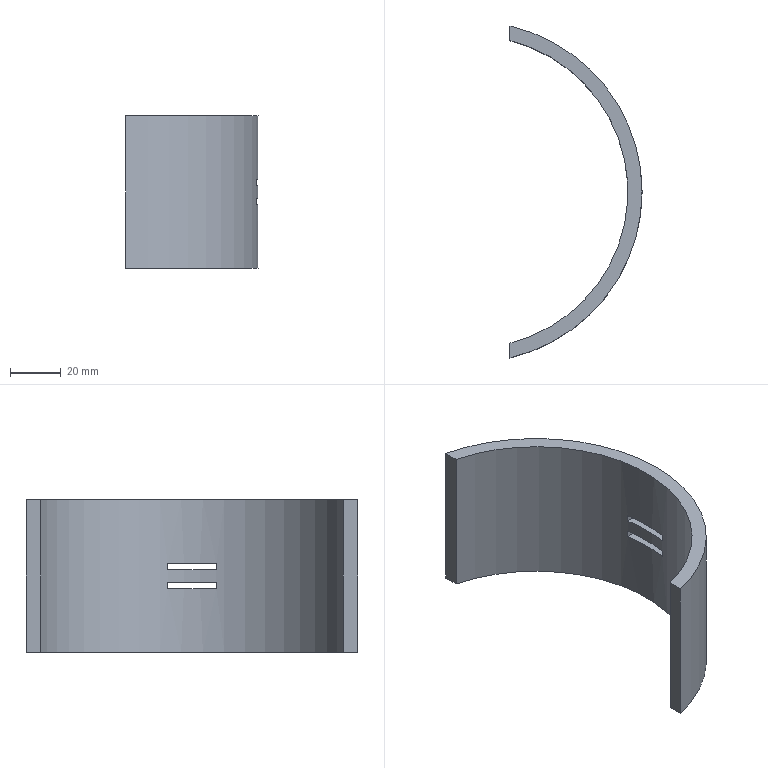Part | SolidWorks | features Extrusion 1, ICE 1 | 1 solid | 14 faces | box 51.978 x 130.553 x 60 mm | volume 56854 mm3 | plane 12 | cylinder 2 | commonest cylinder face diameters 122.792 x1 133.955 x1
STEP:
#1=CARTESIAN_POINT('',(66.293,-9.55,27.496));
#2=VERTEX_POINT('',#1);
#3=CARTESIAN_POINT('',(66.293,-9.55,24.996));
#4=VERTEX_POINT('',#3);
#5=CARTESIAN_POINT('',(66.293,-9.55,60.));
#6=DIRECTION('',(0.,0.,-1.));
#7=VECTOR('',#6,1000.);
#8=LINE('',#5,#7);
#9=EDGE_CURVE('',#2,#4,#8,.T.);
#10=ORIENTED_EDGE('',*,*,#9,.F.);
#11=CARTESIAN_POINT('',(66.293,9.55,27.496));
#12=VERTEX_POINT('',#11);
#13=CARTESIAN_POINT('',(0.,0.,27.496));
#14=DIRECTION('',(0.,0.,-1.));
#15=DIRECTION('',(-1.,0.,0.));
#16=AXIS2_PLACEMENT_3D('',#13,#14,#15);
#17=CIRCLE('',#16,66.978);
#18=EDGE_CURVE('',#12,#2,#17,.T.);
#19=ORIENTED_EDGE('',*,*,#18,.F.);
#20=CARTESIAN_POINT('',(66.293,9.55,24.996));
#21=VERTEX_POINT('',#20);
#22=CARTESIAN_POINT('',(66.293,9.55,60.));
#23=DIRECTION('',(0.,0.,1.));
#24=VECTOR('',#23,1000.);
#25=LINE('',#22,#24);
#26=EDGE_CURVE('',#21,#12,#25,.T.);
#27=ORIENTED_EDGE('',*,*,#26,.F.);
#28=CARTESIAN_POINT('',(0.,0.,24.996));
#29=DIRECTION('',(0.,0.,1.));
#30=DIRECTION('',(1.,0.,0.));
#31=AXIS2_PLACEMENT_3D('',#28,#29,#30);
#32=CIRCLE('',#31,66.978);
#33=EDGE_CURVE('',#4,#21,#32,.T.);
#34=ORIENTED_EDGE('',*,*,#33,.F.);
#35=EDGE_LOOP('',(#10,#19,#27,#34));
#36=FACE_BOUND('',#35,.T.);
#37=CARTESIAN_POINT('',(15.,-65.276,0.));
#38=VERTEX_POINT('',#37);
#39=CARTESIAN_POINT('',(15.,65.276,0.));
#40=VERTEX_POINT('',#39);
#41=CARTESIAN_POINT('',(0.,0.,0.));
#42=DIRECTION('',(0.,0.,1.));
#43=DIRECTION('',(1.,0.,0.));
#44=AXIS2_PLACEMENT_3D('',#41,#42,#43);
#45=CIRCLE('',#44,66.978);
#46=EDGE_CURVE('',#38,#40,#45,.T.);
#47=ORIENTED_EDGE('',*,*,#46,.T.);
#48=CARTESIAN_POINT('',(15.,65.276,60.));
#49=VERTEX_POINT('',#48);
#50=CARTESIAN_POINT('',(15.,65.276,60.));
#51=DIRECTION('',(0.,0.,-1.));
#52=VECTOR('',#51,1000.);
#53=LINE('',#50,#52);
#54=EDGE_CURVE('',#49,#40,#53,.T.);
#55=ORIENTED_EDGE('',*,*,#54,.F.);
#56=CARTESIAN_POINT('',(15.,-65.276,60.));
#57=VERTEX_POINT('',#56);
#58=CARTESIAN_POINT('',(0.,0.,60.));
#59=DIRECTION('',(0.,0.,1.));
#60=DIRECTION('',(1.,0.,0.));
#61=AXIS2_PLACEMENT_3D('',#58,#59,#60);
#62=CIRCLE('',#61,66.978);
#63=EDGE_CURVE('',#57,#49,#62,.T.);
#64=ORIENTED_EDGE('',*,*,#63,.F.);
#65=CARTESIAN_POINT('',(15.,-65.276,60.));
#66=DIRECTION('',(0.,0.,-1.));
#67=VECTOR('',#66,1000.);
#68=LINE('',#65,#67);
#69=EDGE_CURVE('',#57,#38,#68,.T.);
#70=ORIENTED_EDGE('',*,*,#69,.T.);
#71=EDGE_LOOP('',(#47,#55,#64,#70));
#72=FACE_OUTER_BOUND('',#71,.T.);
#73=CARTESIAN_POINT('',(66.293,-9.55,35.004));
#74=VERTEX_POINT('',#73);
#75=CARTESIAN_POINT('',(66.293,-9.55,32.504));
#76=VERTEX_POINT('',#75);
#77=CARTESIAN_POINT('',(66.293,-9.55,60.));
#78=DIRECTION('',(0.,0.,-1.));
#79=VECTOR('',#78,1000.);
#80=LINE('',#77,#79);
#81=EDGE_CURVE('',#74,#76,#80,.T.);
#82=ORIENTED_EDGE('',*,*,#81,.F.);
#83=CARTESIAN_POINT('',(66.293,9.55,35.004));
#84=VERTEX_POINT('',#83);
#85=CARTESIAN_POINT('',(0.,0.,35.004));
#86=DIRECTION('',(0.,0.,-1.));
#87=DIRECTION('',(-1.,0.,0.));
#88=AXIS2_PLACEMENT_3D('',#85,#86,#87);
#89=CIRCLE('',#88,66.978);
#90=EDGE_CURVE('',#84,#74,#89,.T.);
#91=ORIENTED_EDGE('',*,*,#90,.F.);
#92=CARTESIAN_POINT('',(66.293,9.55,32.504));
#93=VERTEX_POINT('',#92);
#94=CARTESIAN_POINT('',(66.293,9.55,60.));
#95=DIRECTION('',(0.,0.,1.));
#96=VECTOR('',#95,1000.);
#97=LINE('',#94,#96);
#98=EDGE_CURVE('',#93,#84,#97,.T.);
#99=ORIENTED_EDGE('',*,*,#98,.F.);
#100=CARTESIAN_POINT('',(0.,0.,32.504));
#101=DIRECTION('',(0.,0.,1.));
#102=DIRECTION('',(1.,0.,0.));
#103=AXIS2_PLACEMENT_3D('',#100,#101,#102);
#104=CIRCLE('',#103,66.978);
#105=EDGE_CURVE('',#76,#93,#104,.T.);
#106=ORIENTED_EDGE('',*,*,#105,.F.);
#107=EDGE_LOOP('',(#82,#91,#99,#106));
#108=FACE_BOUND('',#107,.T.);
#109=CARTESIAN_POINT('',(0.,0.,60.));
#110=DIRECTION('',(0.,0.,-1.));
#111=DIRECTION('',(-1.,0.,0.));
#112=AXIS2_PLACEMENT_3D('',#109,#110,#111);
#113=CYLINDRICAL_SURFACE('',#112,66.978);
#114=ADVANCED_FACE('',(#36,#72,#108),#113,.T.);
#115=CARTESIAN_POINT('',(60.649,-9.55,24.996));
#116=VERTEX_POINT('',#115);
#117=CARTESIAN_POINT('',(60.649,-9.55,27.496));
#118=VERTEX_POINT('',#117);
#119=CARTESIAN_POINT('',(60.649,-9.55,60.));
#120=DIRECTION('',(0.,0.,1.));
#121=VECTOR('',#120,1000.);
#122=LINE('',#119,#121);
#123=EDGE_CURVE('',#116,#118,#122,.T.);
#124=ORIENTED_EDGE('',*,*,#123,.F.);
#125=CARTESIAN_POINT('',(60.649,9.55,24.996));
#126=VERTEX_POINT('',#125);
#127=CARTESIAN_POINT('',(0.,0.,24.996));
#128=DIRECTION('',(0.,0.,-1.));
#129=DIRECTION('',(1.,0.,0.));
#130=AXIS2_PLACEMENT_3D('',#127,#128,#129);
#131=CIRCLE('',#130,61.396);
#132=EDGE_CURVE('',#126,#116,#131,.T.);
#133=ORIENTED_EDGE('',*,*,#132,.F.);
#134=CARTESIAN_POINT('',(60.649,9.55,27.496));
#135=VERTEX_POINT('',#134);
#136=CARTESIAN_POINT('',(60.649,9.55,60.));
#137=DIRECTION('',(0.,0.,-1.));
#138=VECTOR('',#137,1000.);
#139=LINE('',#136,#138);
#140=EDGE_CURVE('',#135,#126,#139,.T.);
#141=ORIENTED_EDGE('',*,*,#140,.F.);
#142=CARTESIAN_POINT('',(0.,0.,27.496));
#143=DIRECTION('',(0.,0.,1.));
#144=DIRECTION('',(-1.,0.,0.));
#145=AXIS2_PLACEMENT_3D('',#142,#143,#144);
#146=CIRCLE('',#145,61.396);
#147=EDGE_CURVE('',#118,#135,#146,.T.);
#148=ORIENTED_EDGE('',*,*,#147,.F.);
#149=EDGE_LOOP('',(#124,#133,#141,#148));
#150=FACE_BOUND('',#149,.T.);
#151=CARTESIAN_POINT('',(15.,59.536,0.));
#152=VERTEX_POINT('',#151);
#153=CARTESIAN_POINT('',(15.,-59.536,0.));
#154=VERTEX_POINT('',#153);
#155=CARTESIAN_POINT('',(0.,0.,0.));
#156=DIRECTION('',(0.,0.,-1.));
#157=DIRECTION('',(1.,0.,0.));
#158=AXIS2_PLACEMENT_3D('',#155,#156,#157);
#159=CIRCLE('',#158,61.396);
#160=EDGE_CURVE('',#152,#154,#159,.T.);
#161=ORIENTED_EDGE('',*,*,#160,.T.);
#162=CARTESIAN_POINT('',(15.,-59.536,60.));
#163=VERTEX_POINT('',#162);
#164=CARTESIAN_POINT('',(15.,-59.536,60.));
#165=DIRECTION('',(0.,0.,-1.));
#166=VECTOR('',#165,1000.);
#167=LINE('',#164,#166);
#168=EDGE_CURVE('',#163,#154,#167,.T.);
#169=ORIENTED_EDGE('',*,*,#168,.F.);
#170=CARTESIAN_POINT('',(15.,59.536,60.));
#171=VERTEX_POINT('',#170);
#172=CARTESIAN_POINT('',(0.,0.,60.));
#173=DIRECTION('',(0.,0.,-1.));
#174=DIRECTION('',(1.,0.,0.));
#175=AXIS2_PLACEMENT_3D('',#172,#173,#174);
#176=CIRCLE('',#175,61.396);
#177=EDGE_CURVE('',#171,#163,#176,.T.);
#178=ORIENTED_EDGE('',*,*,#177,.F.);
#179=CARTESIAN_POINT('',(15.,59.536,60.));
#180=DIRECTION('',(0.,0.,-1.));
#181=VECTOR('',#180,1000.);
#182=LINE('',#179,#181);
#183=EDGE_CURVE('',#171,#152,#182,.T.);
#184=ORIENTED_EDGE('',*,*,#183,.T.);
#185=EDGE_LOOP('',(#161,#169,#178,#184));
#186=FACE_OUTER_BOUND('',#185,.T.);
#187=CARTESIAN_POINT('',(60.649,-9.55,32.504));
#188=VERTEX_POINT('',#187);
#189=CARTESIAN_POINT('',(60.649,-9.55,35.004));
#190=VERTEX_POINT('',#189);
#191=CARTESIAN_POINT('',(60.649,-9.55,60.));
#192=DIRECTION('',(0.,0.,1.));
#193=VECTOR('',#192,1000.);
#194=LINE('',#191,#193);
#195=EDGE_CURVE('',#188,#190,#194,.T.);
#196=ORIENTED_EDGE('',*,*,#195,.F.);
#197=CARTESIAN_POINT('',(60.649,9.55,32.504));
#198=VERTEX_POINT('',#197);
#199=CARTESIAN_POINT('',(0.,0.,32.504));
#200=DIRECTION('',(0.,0.,-1.));
#201=DIRECTION('',(1.,0.,0.));
#202=AXIS2_PLACEMENT_3D('',#199,#200,#201);
#203=CIRCLE('',#202,61.396);
#204=EDGE_CURVE('',#198,#188,#203,.T.);
#205=ORIENTED_EDGE('',*,*,#204,.F.);
#206=CARTESIAN_POINT('',(60.649,9.55,35.004));
#207=VERTEX_POINT('',#206);
#208=CARTESIAN_POINT('',(60.649,9.55,60.));
#209=DIRECTION('',(0.,0.,-1.));
#210=VECTOR('',#209,1000.);
#211=LINE('',#208,#210);
#212=EDGE_CURVE('',#207,#198,#211,.T.);
#213=ORIENTED_EDGE('',*,*,#212,.F.);
#214=CARTESIAN_POINT('',(0.,0.,35.004));
#215=DIRECTION('',(0.,0.,1.));
#216=DIRECTION('',(-1.,0.,0.));
#217=AXIS2_PLACEMENT_3D('',#214,#215,#216);
#218=CIRCLE('',#217,61.396);
#219=EDGE_CURVE('',#190,#207,#218,.T.);
#220=ORIENTED_EDGE('',*,*,#219,.F.);
#221=EDGE_LOOP('',(#196,#205,#213,#220));
#222=FACE_BOUND('',#221,.T.);
#223=CARTESIAN_POINT('',(0.,0.,60.));
#224=DIRECTION('',(0.,0.,-1.));
#225=DIRECTION('',(-1.,0.,0.));
#226=AXIS2_PLACEMENT_3D('',#223,#224,#225);
#227=CYLINDRICAL_SURFACE('',#226,61.396);
#228=ADVANCED_FACE('',(#150,#186,#222),#227,.F.);
#229=CARTESIAN_POINT('',(15.,65.276,0.));
#230=DIRECTION('',(0.,-1.,0.));
#231=VECTOR('',#230,1000.);
#232=LINE('',#229,#231);
#233=EDGE_CURVE('',#40,#152,#232,.T.);
#234=ORIENTED_EDGE('',*,*,#233,.T.);
#235=ORIENTED_EDGE('',*,*,#183,.F.);
#236=CARTESIAN_POINT('',(15.,65.276,60.));
#237=DIRECTION('',(0.,-1.,0.));
#238=VECTOR('',#237,1000.);
#239=LINE('',#236,#238);
#240=EDGE_CURVE('',#49,#171,#239,.T.);
#241=ORIENTED_EDGE('',*,*,#240,.F.);
#242=ORIENTED_EDGE('',*,*,#54,.T.);
#243=EDGE_LOOP('',(#234,#235,#241,#242));
#244=FACE_OUTER_BOUND('',#243,.T.);
#245=CARTESIAN_POINT('',(15.,65.276,60.));
#246=DIRECTION('',(1.,0.,0.));
#247=DIRECTION('',(0.,0.,-1.));
#248=AXIS2_PLACEMENT_3D('',#245,#246,#247);
#249=PLANE('',#248);
#250=ADVANCED_FACE('',(#244),#249,.F.);
#251=CARTESIAN_POINT('',(15.,-59.536,0.));
#252=DIRECTION('',(0.,-1.,0.));
#253=VECTOR('',#252,1000.);
#254=LINE('',#251,#253);
#255=EDGE_CURVE('',#154,#38,#254,.T.);
#256=ORIENTED_EDGE('',*,*,#255,.T.);
#257=ORIENTED_EDGE('',*,*,#69,.F.);
#258=CARTESIAN_POINT('',(15.,-59.536,60.));
#259=DIRECTION('',(0.,-1.,0.));
#260=VECTOR('',#259,1000.);
#261=LINE('',#258,#260);
#262=EDGE_CURVE('',#163,#57,#261,.T.);
#263=ORIENTED_EDGE('',*,*,#262,.F.);
#264=ORIENTED_EDGE('',*,*,#168,.T.);
#265=EDGE_LOOP('',(#256,#257,#263,#264));
#266=FACE_OUTER_BOUND('',#265,.T.);
#267=CARTESIAN_POINT('',(15.,-59.536,60.));
#268=DIRECTION('',(1.,0.,0.));
#269=DIRECTION('',(0.,0.,-1.));
#270=AXIS2_PLACEMENT_3D('',#267,#268,#269);
#271=PLANE('',#270);
#272=ADVANCED_FACE('',(#266),#271,.F.);
#273=ORIENTED_EDGE('',*,*,#63,.T.);
#274=ORIENTED_EDGE('',*,*,#240,.T.);
#275=ORIENTED_EDGE('',*,*,#177,.T.);
#276=ORIENTED_EDGE('',*,*,#262,.T.);
#277=EDGE_LOOP('',(#273,#274,#275,#276));
#278=FACE_OUTER_BOUND('',#277,.T.);
#279=CARTESIAN_POINT('',(0.,0.,60.));
#280=DIRECTION('',(0.,0.,1.));
#281=DIRECTION('',(1.,0.,0.));
#282=AXIS2_PLACEMENT_3D('',#279,#280,#281);
#283=PLANE('',#282);
#284=ADVANCED_FACE('',(#278),#283,.T.);
#285=ORIENTED_EDGE('',*,*,#46,.F.);
#286=ORIENTED_EDGE('',*,*,#255,.F.);
#287=ORIENTED_EDGE('',*,*,#160,.F.);
#288=ORIENTED_EDGE('',*,*,#233,.F.);
#289=EDGE_LOOP('',(#285,#286,#287,#288));
#290=FACE_OUTER_BOUND('',#289,.T.);
#291=CARTESIAN_POINT('',(0.,0.,0.));
#292=DIRECTION('',(0.,0.,1.));
#293=DIRECTION('',(1.,0.,0.));
#294=AXIS2_PLACEMENT_3D('',#291,#292,#293);
#295=PLANE('',#294);
#296=ADVANCED_FACE('',(#290),#295,.F.);
#297=ORIENTED_EDGE('',*,*,#9,.T.);
#298=CARTESIAN_POINT('',(115.,-9.55,24.996));
#299=DIRECTION('',(-1.,0.,0.));
#300=VECTOR('',#299,1000.);
#301=LINE('',#298,#300);
#302=EDGE_CURVE('',#4,#116,#301,.T.);
#303=ORIENTED_EDGE('',*,*,#302,.T.);
#304=ORIENTED_EDGE('',*,*,#123,.T.);
#305=CARTESIAN_POINT('',(115.,-9.55,27.496));
#306=DIRECTION('',(-1.,0.,0.));
#307=VECTOR('',#306,1000.);
#308=LINE('',#305,#307);
#309=EDGE_CURVE('',#2,#118,#308,.T.);
#310=ORIENTED_EDGE('',*,*,#309,.F.);
#311=EDGE_LOOP('',(#297,#303,#304,#310));
#312=FACE_OUTER_BOUND('',#311,.T.);
#313=CARTESIAN_POINT('',(115.,-9.55,27.496));
#314=DIRECTION('',(0.,1.,0.));
#315=DIRECTION('',(0.,0.,1.));
#316=AXIS2_PLACEMENT_3D('',#313,#314,#315);
#317=PLANE('',#316);
#318=ADVANCED_FACE('',(#312),#317,.T.);
#319=ORIENTED_EDGE('',*,*,#33,.T.);
#320=CARTESIAN_POINT('',(115.,9.55,24.996));
#321=DIRECTION('',(-1.,0.,0.));
#322=VECTOR('',#321,1000.);
#323=LINE('',#320,#322);
#324=EDGE_CURVE('',#21,#126,#323,.T.);
#325=ORIENTED_EDGE('',*,*,#324,.T.);
#326=ORIENTED_EDGE('',*,*,#132,.T.);
#327=ORIENTED_EDGE('',*,*,#302,.F.);
#328=EDGE_LOOP('',(#319,#325,#326,#327));
#329=FACE_OUTER_BOUND('',#328,.T.);
#330=CARTESIAN_POINT('',(115.,9.55,24.996));
#331=DIRECTION('',(0.,0.,1.));
#332=DIRECTION('',(1.,0.,0.));
#333=AXIS2_PLACEMENT_3D('',#330,#331,#332);
#334=PLANE('',#333);
#335=ADVANCED_FACE('',(#329),#334,.T.);
#336=ORIENTED_EDGE('',*,*,#26,.T.);
#337=CARTESIAN_POINT('',(115.,9.55,27.496));
#338=DIRECTION('',(-1.,0.,0.));
#339=VECTOR('',#338,1000.);
#340=LINE('',#337,#339);
#341=EDGE_CURVE('',#12,#135,#340,.T.);
#342=ORIENTED_EDGE('',*,*,#341,.T.);
#343=ORIENTED_EDGE('',*,*,#140,.T.);
#344=ORIENTED_EDGE('',*,*,#324,.F.);
#345=EDGE_LOOP('',(#336,#342,#343,#344));
#346=FACE_OUTER_BOUND('',#345,.T.);
#347=CARTESIAN_POINT('',(115.,9.55,27.496));
#348=DIRECTION('',(0.,-1.,0.));
#349=DIRECTION('',(0.,0.,-1.));
#350=AXIS2_PLACEMENT_3D('',#347,#348,#349);
#351=PLANE('',#350);
#352=ADVANCED_FACE('',(#346),#351,.T.);
#353=ORIENTED_EDGE('',*,*,#18,.T.);
#354=ORIENTED_EDGE('',*,*,#309,.T.);
#355=ORIENTED_EDGE('',*,*,#147,.T.);
#356=ORIENTED_EDGE('',*,*,#341,.F.);
#357=EDGE_LOOP('',(#353,#354,#355,#356));
#358=FACE_OUTER_BOUND('',#357,.T.);
#359=CARTESIAN_POINT('',(115.,-9.55,27.496));
#360=DIRECTION('',(0.,0.,-1.));
#361=DIRECTION('',(-1.,0.,0.));
#362=AXIS2_PLACEMENT_3D('',#359,#360,#361);
#363=PLANE('',#362);
#364=ADVANCED_FACE('',(#358),#363,.T.);
#365=ORIENTED_EDGE('',*,*,#81,.T.);
#366=CARTESIAN_POINT('',(115.,-9.55,32.504));
#367=DIRECTION('',(-1.,0.,0.));
#368=VECTOR('',#367,1000.);
#369=LINE('',#366,#368);
#370=EDGE_CURVE('',#76,#188,#369,.T.);
#371=ORIENTED_EDGE('',*,*,#370,.T.);
#372=ORIENTED_EDGE('',*,*,#195,.T.);
#373=CARTESIAN_POINT('',(115.,-9.55,35.004));
#374=DIRECTION('',(-1.,0.,0.));
#375=VECTOR('',#374,1000.);
#376=LINE('',#373,#375);
#377=EDGE_CURVE('',#74,#190,#376,.T.);
#378=ORIENTED_EDGE('',*,*,#377,.F.);
#379=EDGE_LOOP('',(#365,#371,#372,#378));
#380=FACE_OUTER_BOUND('',#379,.T.);
#381=CARTESIAN_POINT('',(115.,-9.55,32.504));
#382=DIRECTION('',(0.,1.,0.));
#383=DIRECTION('',(0.,0.,1.));
#384=AXIS2_PLACEMENT_3D('',#381,#382,#383);
#385=PLANE('',#384);
#386=ADVANCED_FACE('',(#380),#385,.T.);
#387=ORIENTED_EDGE('',*,*,#105,.T.);
#388=CARTESIAN_POINT('',(115.,9.55,32.504));
#389=DIRECTION('',(-1.,0.,0.));
#390=VECTOR('',#389,1000.);
#391=LINE('',#388,#390);
#392=EDGE_CURVE('',#93,#198,#391,.T.);
#393=ORIENTED_EDGE('',*,*,#392,.T.);
#394=ORIENTED_EDGE('',*,*,#204,.T.);
#395=ORIENTED_EDGE('',*,*,#370,.F.);
#396=EDGE_LOOP('',(#387,#393,#394,#395));
#397=FACE_OUTER_BOUND('',#396,.T.);
#398=CARTESIAN_POINT('',(115.,-9.55,32.504));
#399=DIRECTION('',(0.,0.,1.));
#400=DIRECTION('',(1.,0.,0.));
#401=AXIS2_PLACEMENT_3D('',#398,#399,#400);
#402=PLANE('',#401);
#403=ADVANCED_FACE('',(#397),#402,.T.);
#404=ORIENTED_EDGE('',*,*,#98,.T.);
#405=CARTESIAN_POINT('',(115.,9.55,35.004));
#406=DIRECTION('',(-1.,0.,0.));
#407=VECTOR('',#406,1000.);
#408=LINE('',#405,#407);
#409=EDGE_CURVE('',#84,#207,#408,.T.);
#410=ORIENTED_EDGE('',*,*,#409,.T.);
#411=ORIENTED_EDGE('',*,*,#212,.T.);
#412=ORIENTED_EDGE('',*,*,#392,.F.);
#413=EDGE_LOOP('',(#404,#410,#411,#412));
#414=FACE_OUTER_BOUND('',#413,.T.);
#415=CARTESIAN_POINT('',(115.,9.55,32.504));
#416=DIRECTION('',(0.,-1.,0.));
#417=DIRECTION('',(0.,0.,-1.));
#418=AXIS2_PLACEMENT_3D('',#415,#416,#417);
#419=PLANE('',#418);
#420=ADVANCED_FACE('',(#414),#419,.T.);
#421=ORIENTED_EDGE('',*,*,#90,.T.);
#422=ORIENTED_EDGE('',*,*,#377,.T.);
#423=ORIENTED_EDGE('',*,*,#219,.T.);
#424=ORIENTED_EDGE('',*,*,#409,.F.);
#425=EDGE_LOOP('',(#421,#422,#423,#424));
#426=FACE_OUTER_BOUND('',#425,.T.);
#427=CARTESIAN_POINT('',(115.,9.55,35.004));
#428=DIRECTION('',(0.,0.,-1.));
#429=DIRECTION('',(-1.,0.,0.));
#430=AXIS2_PLACEMENT_3D('',#427,#428,#429);
#431=PLANE('',#430);
#432=ADVANCED_FACE('',(#426),#431,.T.);
#433=CLOSED_SHELL('',(#114,#228,#250,#272,#284,#296,#318,#335,#352,#364,#386,#403,#420,#432));
#434=MANIFOLD_SOLID_BREP('',#433);
#435=CARTESIAN_POINT('',(0.,0.,0.));
#436=DIRECTION('',(0.,0.,1.));
#437=DIRECTION('',(1.,0.,0.));
#438=AXIS2_PLACEMENT_3D('',#435,#436,#437);
#439=(LENGTH_UNIT()NAMED_UNIT(*)SI_UNIT(.MILLI.,.METRE.));
#440=UNCERTAINTY_MEASURE_WITH_UNIT(LENGTH_MEASURE(0.00001),#439,'','');
#441=(NAMED_UNIT(*)PLANE_ANGLE_UNIT()SI_UNIT($,.RADIAN.));
#442=(NAMED_UNIT(*)SI_UNIT($,.STERADIAN.)SOLID_ANGLE_UNIT());
#443=(GEOMETRIC_REPRESENTATION_CONTEXT(3)GLOBAL_UNCERTAINTY_ASSIGNED_CONTEXT((#440))GLOBAL_UNIT_ASSIGNED_CONTEXT((#439,#441,#442))REPRESENTATION_CONTEXT('',''));
#444=ADVANCED_BREP_SHAPE_REPRESENTATION('',(#434,#438),#443);